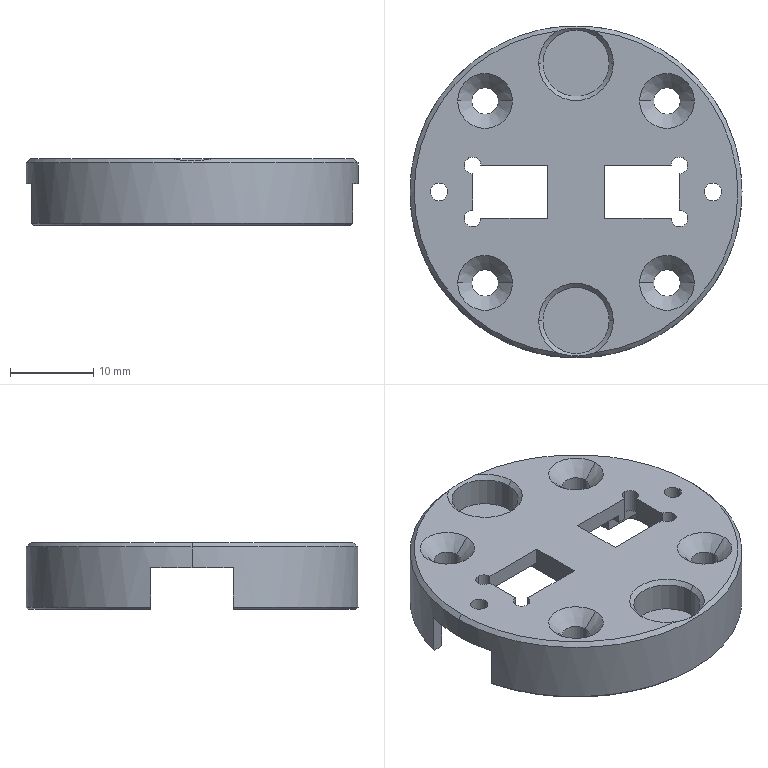Part | NX | features BREP 1 | 1 solid | 86 faces | box 40 x 40 x 8 mm | volume 4406 mm3 | cylinder 32 | plane 32 | cone 22 | commonest cylinder face diameters 2 x12 3.2 x8 2.1 x4 8 x4 37.04 x2 40 x2